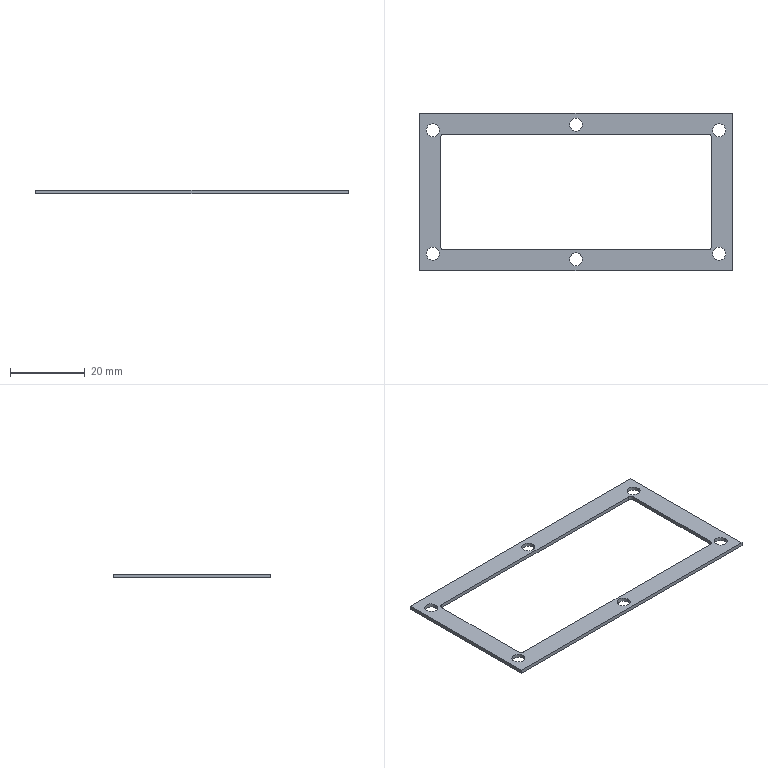Part | SolidWorks | features Extrusion 1, Fillet 1 | 1 solid | 26 faces | box 83.5 x 42 x 1 mm | volume 1203 mm3 | cylinder 16 | plane 10 | commonest cylinder face diameters 3.5 x12 2 x4
STEP:
#1=CARTESIAN_POINT('',(-1.75,-18.,1.));
#2=VERTEX_POINT('',#1);
#3=CARTESIAN_POINT('',(1.75,-18.,1.));
#4=VERTEX_POINT('',#3);
#5=CARTESIAN_POINT('',(0.,-18.,1.));
#6=DIRECTION('',(0.,0.,1.));
#7=DIRECTION('',(1.,0.,0.));
#8=AXIS2_PLACEMENT_3D('',#5,#6,#7);
#9=CIRCLE('',#8,1.75);
#10=EDGE_CURVE('',#2,#4,#9,.T.);
#11=ORIENTED_EDGE('',*,*,#10,.T.);
#12=CARTESIAN_POINT('',(1.75,-18.,0.));
#13=VERTEX_POINT('',#12);
#14=CARTESIAN_POINT('',(1.75,-18.,1.));
#15=DIRECTION('',(0.,0.,-1.));
#16=VECTOR('',#15,1000.);
#17=LINE('',#14,#16);
#18=EDGE_CURVE('',#4,#13,#17,.T.);
#19=ORIENTED_EDGE('',*,*,#18,.T.);
#20=CARTESIAN_POINT('',(-1.75,-18.,0.));
#21=VERTEX_POINT('',#20);
#22=CARTESIAN_POINT('',(0.,-18.,0.));
#23=DIRECTION('',(0.,0.,1.));
#24=DIRECTION('',(1.,0.,0.));
#25=AXIS2_PLACEMENT_3D('',#22,#23,#24);
#26=CIRCLE('',#25,1.75);
#27=EDGE_CURVE('',#21,#13,#26,.T.);
#28=ORIENTED_EDGE('',*,*,#27,.F.);
#29=CARTESIAN_POINT('',(-1.75,-18.,1.));
#30=DIRECTION('',(0.,0.,-1.));
#31=VECTOR('',#30,1000.);
#32=LINE('',#29,#31);
#33=EDGE_CURVE('',#2,#21,#32,.T.);
#34=ORIENTED_EDGE('',*,*,#33,.F.);
#35=EDGE_LOOP('',(#11,#19,#28,#34));
#36=FACE_OUTER_BOUND('',#35,.T.);
#37=CARTESIAN_POINT('',(0.,-18.,1.));
#38=DIRECTION('',(0.,0.,-1.));
#39=DIRECTION('',(-1.,0.,0.));
#40=AXIS2_PLACEMENT_3D('',#37,#38,#39);
#41=CYLINDRICAL_SURFACE('',#40,1.75);
#42=ADVANCED_FACE('',(#36),#41,.F.);
#43=CARTESIAN_POINT('',(-1.75,18.,1.));
#44=VERTEX_POINT('',#43);
#45=CARTESIAN_POINT('',(1.75,18.,1.));
#46=VERTEX_POINT('',#45);
#47=CARTESIAN_POINT('',(0.,18.,1.));
#48=DIRECTION('',(0.,0.,1.));
#49=DIRECTION('',(1.,0.,0.));
#50=AXIS2_PLACEMENT_3D('',#47,#48,#49);
#51=CIRCLE('',#50,1.75);
#52=EDGE_CURVE('',#44,#46,#51,.T.);
#53=ORIENTED_EDGE('',*,*,#52,.T.);
#54=CARTESIAN_POINT('',(1.75,18.,0.));
#55=VERTEX_POINT('',#54);
#56=CARTESIAN_POINT('',(1.75,18.,1.));
#57=DIRECTION('',(0.,0.,-1.));
#58=VECTOR('',#57,1000.);
#59=LINE('',#56,#58);
#60=EDGE_CURVE('',#46,#55,#59,.T.);
#61=ORIENTED_EDGE('',*,*,#60,.T.);
#62=CARTESIAN_POINT('',(-1.75,18.,0.));
#63=VERTEX_POINT('',#62);
#64=CARTESIAN_POINT('',(0.,18.,0.));
#65=DIRECTION('',(0.,0.,1.));
#66=DIRECTION('',(1.,0.,0.));
#67=AXIS2_PLACEMENT_3D('',#64,#65,#66);
#68=CIRCLE('',#67,1.75);
#69=EDGE_CURVE('',#63,#55,#68,.T.);
#70=ORIENTED_EDGE('',*,*,#69,.F.);
#71=CARTESIAN_POINT('',(-1.75,18.,1.));
#72=DIRECTION('',(0.,0.,-1.));
#73=VECTOR('',#72,1000.);
#74=LINE('',#71,#73);
#75=EDGE_CURVE('',#44,#63,#74,.T.);
#76=ORIENTED_EDGE('',*,*,#75,.F.);
#77=EDGE_LOOP('',(#53,#61,#70,#76));
#78=FACE_OUTER_BOUND('',#77,.T.);
#79=CARTESIAN_POINT('',(0.,18.,1.));
#80=DIRECTION('',(0.,0.,-1.));
#81=DIRECTION('',(-1.,0.,0.));
#82=AXIS2_PLACEMENT_3D('',#79,#80,#81);
#83=CYLINDRICAL_SURFACE('',#82,1.75);
#84=ADVANCED_FACE('',(#78),#83,.F.);
#85=CARTESIAN_POINT('',(-40.,-16.5,1.));
#86=VERTEX_POINT('',#85);
#87=CARTESIAN_POINT('',(-36.5,-16.5,1.));
#88=VERTEX_POINT('',#87);
#89=CARTESIAN_POINT('',(-38.25,-16.5,1.));
#90=DIRECTION('',(0.,0.,1.));
#91=DIRECTION('',(1.,0.,0.));
#92=AXIS2_PLACEMENT_3D('',#89,#90,#91);
#93=CIRCLE('',#92,1.75);
#94=EDGE_CURVE('',#86,#88,#93,.T.);
#95=ORIENTED_EDGE('',*,*,#94,.T.);
#96=CARTESIAN_POINT('',(-36.5,-16.5,0.));
#97=VERTEX_POINT('',#96);
#98=CARTESIAN_POINT('',(-36.5,-16.5,1.));
#99=DIRECTION('',(0.,0.,-1.));
#100=VECTOR('',#99,1000.);
#101=LINE('',#98,#100);
#102=EDGE_CURVE('',#88,#97,#101,.T.);
#103=ORIENTED_EDGE('',*,*,#102,.T.);
#104=CARTESIAN_POINT('',(-40.,-16.5,0.));
#105=VERTEX_POINT('',#104);
#106=CARTESIAN_POINT('',(-38.25,-16.5,0.));
#107=DIRECTION('',(0.,0.,1.));
#108=DIRECTION('',(1.,0.,0.));
#109=AXIS2_PLACEMENT_3D('',#106,#107,#108);
#110=CIRCLE('',#109,1.75);
#111=EDGE_CURVE('',#105,#97,#110,.T.);
#112=ORIENTED_EDGE('',*,*,#111,.F.);
#113=CARTESIAN_POINT('',(-40.,-16.5,1.));
#114=DIRECTION('',(0.,0.,-1.));
#115=VECTOR('',#114,1000.);
#116=LINE('',#113,#115);
#117=EDGE_CURVE('',#86,#105,#116,.T.);
#118=ORIENTED_EDGE('',*,*,#117,.F.);
#119=EDGE_LOOP('',(#95,#103,#112,#118));
#120=FACE_OUTER_BOUND('',#119,.T.);
#121=CARTESIAN_POINT('',(-38.25,-16.5,1.));
#122=DIRECTION('',(0.,0.,-1.));
#123=DIRECTION('',(-1.,0.,0.));
#124=AXIS2_PLACEMENT_3D('',#121,#122,#123);
#125=CYLINDRICAL_SURFACE('',#124,1.75);
#126=ADVANCED_FACE('',(#120),#125,.F.);
#127=CARTESIAN_POINT('',(36.5,-16.5,1.));
#128=VERTEX_POINT('',#127);
#129=CARTESIAN_POINT('',(40.,-16.5,1.));
#130=VERTEX_POINT('',#129);
#131=CARTESIAN_POINT('',(38.25,-16.5,1.));
#132=DIRECTION('',(0.,0.,1.));
#133=DIRECTION('',(1.,0.,0.));
#134=AXIS2_PLACEMENT_3D('',#131,#132,#133);
#135=CIRCLE('',#134,1.75);
#136=EDGE_CURVE('',#128,#130,#135,.T.);
#137=ORIENTED_EDGE('',*,*,#136,.T.);
#138=CARTESIAN_POINT('',(40.,-16.5,0.));
#139=VERTEX_POINT('',#138);
#140=CARTESIAN_POINT('',(40.,-16.5,1.));
#141=DIRECTION('',(0.,0.,-1.));
#142=VECTOR('',#141,1000.);
#143=LINE('',#140,#142);
#144=EDGE_CURVE('',#130,#139,#143,.T.);
#145=ORIENTED_EDGE('',*,*,#144,.T.);
#146=CARTESIAN_POINT('',(36.5,-16.5,0.));
#147=VERTEX_POINT('',#146);
#148=CARTESIAN_POINT('',(38.25,-16.5,0.));
#149=DIRECTION('',(0.,0.,1.));
#150=DIRECTION('',(1.,0.,0.));
#151=AXIS2_PLACEMENT_3D('',#148,#149,#150);
#152=CIRCLE('',#151,1.75);
#153=EDGE_CURVE('',#147,#139,#152,.T.);
#154=ORIENTED_EDGE('',*,*,#153,.F.);
#155=CARTESIAN_POINT('',(36.5,-16.5,1.));
#156=DIRECTION('',(0.,0.,-1.));
#157=VECTOR('',#156,1000.);
#158=LINE('',#155,#157);
#159=EDGE_CURVE('',#128,#147,#158,.T.);
#160=ORIENTED_EDGE('',*,*,#159,.F.);
#161=EDGE_LOOP('',(#137,#145,#154,#160));
#162=FACE_OUTER_BOUND('',#161,.T.);
#163=CARTESIAN_POINT('',(38.25,-16.5,1.));
#164=DIRECTION('',(0.,0.,-1.));
#165=DIRECTION('',(-1.,0.,0.));
#166=AXIS2_PLACEMENT_3D('',#163,#164,#165);
#167=CYLINDRICAL_SURFACE('',#166,1.75);
#168=ADVANCED_FACE('',(#162),#167,.F.);
#169=CARTESIAN_POINT('',(36.5,16.5,1.));
#170=VERTEX_POINT('',#169);
#171=CARTESIAN_POINT('',(40.,16.5,1.));
#172=VERTEX_POINT('',#171);
#173=CARTESIAN_POINT('',(38.25,16.5,1.));
#174=DIRECTION('',(0.,0.,1.));
#175=DIRECTION('',(1.,0.,0.));
#176=AXIS2_PLACEMENT_3D('',#173,#174,#175);
#177=CIRCLE('',#176,1.75);
#178=EDGE_CURVE('',#170,#172,#177,.T.);
#179=ORIENTED_EDGE('',*,*,#178,.T.);
#180=CARTESIAN_POINT('',(40.,16.5,0.));
#181=VERTEX_POINT('',#180);
#182=CARTESIAN_POINT('',(40.,16.5,1.));
#183=DIRECTION('',(0.,0.,-1.));
#184=VECTOR('',#183,1000.);
#185=LINE('',#182,#184);
#186=EDGE_CURVE('',#172,#181,#185,.T.);
#187=ORIENTED_EDGE('',*,*,#186,.T.);
#188=CARTESIAN_POINT('',(36.5,16.5,0.));
#189=VERTEX_POINT('',#188);
#190=CARTESIAN_POINT('',(38.25,16.5,0.));
#191=DIRECTION('',(0.,0.,1.));
#192=DIRECTION('',(1.,0.,0.));
#193=AXIS2_PLACEMENT_3D('',#190,#191,#192);
#194=CIRCLE('',#193,1.75);
#195=EDGE_CURVE('',#189,#181,#194,.T.);
#196=ORIENTED_EDGE('',*,*,#195,.F.);
#197=CARTESIAN_POINT('',(36.5,16.5,1.));
#198=DIRECTION('',(0.,0.,-1.));
#199=VECTOR('',#198,1000.);
#200=LINE('',#197,#199);
#201=EDGE_CURVE('',#170,#189,#200,.T.);
#202=ORIENTED_EDGE('',*,*,#201,.F.);
#203=EDGE_LOOP('',(#179,#187,#196,#202));
#204=FACE_OUTER_BOUND('',#203,.T.);
#205=CARTESIAN_POINT('',(38.25,16.5,1.));
#206=DIRECTION('',(0.,0.,-1.));
#207=DIRECTION('',(-1.,0.,0.));
#208=AXIS2_PLACEMENT_3D('',#205,#206,#207);
#209=CYLINDRICAL_SURFACE('',#208,1.75);
#210=ADVANCED_FACE('',(#204),#209,.F.);
#211=CARTESIAN_POINT('',(-40.,16.5,1.));
#212=VERTEX_POINT('',#211);
#213=CARTESIAN_POINT('',(-36.5,16.5,1.));
#214=VERTEX_POINT('',#213);
#215=CARTESIAN_POINT('',(-38.25,16.5,1.));
#216=DIRECTION('',(0.,0.,1.));
#217=DIRECTION('',(1.,0.,0.));
#218=AXIS2_PLACEMENT_3D('',#215,#216,#217);
#219=CIRCLE('',#218,1.75);
#220=EDGE_CURVE('',#212,#214,#219,.T.);
#221=ORIENTED_EDGE('',*,*,#220,.T.);
#222=CARTESIAN_POINT('',(-36.5,16.5,0.));
#223=VERTEX_POINT('',#222);
#224=CARTESIAN_POINT('',(-36.5,16.5,1.));
#225=DIRECTION('',(0.,0.,-1.));
#226=VECTOR('',#225,1000.);
#227=LINE('',#224,#226);
#228=EDGE_CURVE('',#214,#223,#227,.T.);
#229=ORIENTED_EDGE('',*,*,#228,.T.);
#230=CARTESIAN_POINT('',(-40.,16.5,0.));
#231=VERTEX_POINT('',#230);
#232=CARTESIAN_POINT('',(-38.25,16.5,0.));
#233=DIRECTION('',(0.,0.,1.));
#234=DIRECTION('',(1.,0.,0.));
#235=AXIS2_PLACEMENT_3D('',#232,#233,#234);
#236=CIRCLE('',#235,1.75);
#237=EDGE_CURVE('',#231,#223,#236,.T.);
#238=ORIENTED_EDGE('',*,*,#237,.F.);
#239=CARTESIAN_POINT('',(-40.,16.5,1.));
#240=DIRECTION('',(0.,0.,-1.));
#241=VECTOR('',#240,1000.);
#242=LINE('',#239,#241);
#243=EDGE_CURVE('',#212,#231,#242,.T.);
#244=ORIENTED_EDGE('',*,*,#243,.F.);
#245=EDGE_LOOP('',(#221,#229,#238,#244));
#246=FACE_OUTER_BOUND('',#245,.T.);
#247=CARTESIAN_POINT('',(-38.25,16.5,1.));
#248=DIRECTION('',(0.,0.,-1.));
#249=DIRECTION('',(-1.,0.,0.));
#250=AXIS2_PLACEMENT_3D('',#247,#248,#249);
#251=CYLINDRICAL_SURFACE('',#250,1.75);
#252=ADVANCED_FACE('',(#246),#251,.F.);
#253=ORIENTED_EDGE('',*,*,#52,.F.);
#254=CARTESIAN_POINT('',(0.,18.,1.));
#255=DIRECTION('',(0.,0.,1.));
#256=DIRECTION('',(1.,0.,0.));
#257=AXIS2_PLACEMENT_3D('',#254,#255,#256);
#258=CIRCLE('',#257,1.75);
#259=EDGE_CURVE('',#46,#44,#258,.T.);
#260=ORIENTED_EDGE('',*,*,#259,.F.);
#261=EDGE_LOOP('',(#253,#260));
#262=FACE_BOUND('',#261,.T.);
#263=ORIENTED_EDGE('',*,*,#136,.F.);
#264=CARTESIAN_POINT('',(38.25,-16.5,1.));
#265=DIRECTION('',(0.,0.,1.));
#266=DIRECTION('',(1.,0.,0.));
#267=AXIS2_PLACEMENT_3D('',#264,#265,#266);
#268=CIRCLE('',#267,1.75);
#269=EDGE_CURVE('',#130,#128,#268,.T.);
#270=ORIENTED_EDGE('',*,*,#269,.F.);
#271=EDGE_LOOP('',(#263,#270));
#272=FACE_BOUND('',#271,.T.);
#273=ORIENTED_EDGE('',*,*,#220,.F.);
#274=CARTESIAN_POINT('',(-38.25,16.5,1.));
#275=DIRECTION('',(0.,0.,1.));
#276=DIRECTION('',(1.,0.,0.));
#277=AXIS2_PLACEMENT_3D('',#274,#275,#276);
#278=CIRCLE('',#277,1.75);
#279=EDGE_CURVE('',#214,#212,#278,.T.);
#280=ORIENTED_EDGE('',*,*,#279,.F.);
#281=EDGE_LOOP('',(#273,#280));
#282=FACE_BOUND('',#281,.T.);
#283=CARTESIAN_POINT('',(-41.75,21.,1.));
#284=VERTEX_POINT('',#283);
#285=CARTESIAN_POINT('',(-41.75,-21.,1.));
#286=VERTEX_POINT('',#285);
#287=CARTESIAN_POINT('',(-41.75,-21.,1.));
#288=DIRECTION('',(0.,-1.,0.));
#289=VECTOR('',#288,1000.);
#290=LINE('',#287,#289);
#291=EDGE_CURVE('',#284,#286,#290,.T.);
#292=ORIENTED_EDGE('',*,*,#291,.T.);
#293=CARTESIAN_POINT('',(41.75,-21.,1.));
#294=VERTEX_POINT('',#293);
#295=CARTESIAN_POINT('',(41.75,-21.,1.));
#296=DIRECTION('',(1.,0.,0.));
#297=VECTOR('',#296,1000.);
#298=LINE('',#295,#297);
#299=EDGE_CURVE('',#286,#294,#298,.T.);
#300=ORIENTED_EDGE('',*,*,#299,.T.);
#301=CARTESIAN_POINT('',(41.75,21.,1.));
#302=VERTEX_POINT('',#301);
#303=CARTESIAN_POINT('',(41.75,-21.,1.));
#304=DIRECTION('',(0.,1.,0.));
#305=VECTOR('',#304,1000.);
#306=LINE('',#303,#305);
#307=EDGE_CURVE('',#294,#302,#306,.T.);
#308=ORIENTED_EDGE('',*,*,#307,.T.);
#309=CARTESIAN_POINT('',(41.75,21.,1.));
#310=DIRECTION('',(-1.,0.,0.));
#311=VECTOR('',#310,1000.);
#312=LINE('',#309,#311);
#313=EDGE_CURVE('',#302,#284,#312,.T.);
#314=ORIENTED_EDGE('',*,*,#313,.T.);
#315=EDGE_LOOP('',(#292,#300,#308,#314));
#316=FACE_OUTER_BOUND('',#315,.T.);
#317=ORIENTED_EDGE('',*,*,#178,.F.);
#318=CARTESIAN_POINT('',(38.25,16.5,1.));
#319=DIRECTION('',(0.,0.,1.));
#320=DIRECTION('',(1.,0.,0.));
#321=AXIS2_PLACEMENT_3D('',#318,#319,#320);
#322=CIRCLE('',#321,1.75);
#323=EDGE_CURVE('',#172,#170,#322,.T.);
#324=ORIENTED_EDGE('',*,*,#323,.F.);
#325=EDGE_LOOP('',(#317,#324));
#326=FACE_BOUND('',#325,.T.);
#327=ORIENTED_EDGE('',*,*,#94,.F.);
#328=CARTESIAN_POINT('',(-38.25,-16.5,1.));
#329=DIRECTION('',(0.,0.,1.));
#330=DIRECTION('',(1.,0.,0.));
#331=AXIS2_PLACEMENT_3D('',#328,#329,#330);
#332=CIRCLE('',#331,1.75);
#333=EDGE_CURVE('',#88,#86,#332,.T.);
#334=ORIENTED_EDGE('',*,*,#333,.F.);
#335=EDGE_LOOP('',(#327,#334));
#336=FACE_BOUND('',#335,.T.);
#337=ORIENTED_EDGE('',*,*,#10,.F.);
#338=CARTESIAN_POINT('',(0.,-18.,1.));
#339=DIRECTION('',(0.,0.,1.));
#340=DIRECTION('',(1.,0.,0.));
#341=AXIS2_PLACEMENT_3D('',#338,#339,#340);
#342=CIRCLE('',#341,1.75);
#343=EDGE_CURVE('',#4,#2,#342,.T.);
#344=ORIENTED_EDGE('',*,*,#343,.F.);
#345=EDGE_LOOP('',(#337,#344));
#346=FACE_BOUND('',#345,.T.);
#347=CARTESIAN_POINT('',(-35.25,-15.5,1.));
#348=VERTEX_POINT('',#347);
#349=CARTESIAN_POINT('',(35.25,-15.5,1.));
#350=VERTEX_POINT('',#349);
#351=CARTESIAN_POINT('',(36.25,-15.5,1.));
#352=DIRECTION('',(1.,0.,0.));
#353=VECTOR('',#352,1000.);
#354=LINE('',#351,#353);
#355=EDGE_CURVE('',#348,#350,#354,.T.);
#356=ORIENTED_EDGE('',*,*,#355,.F.);
#357=CARTESIAN_POINT('',(-36.25,-14.5,1.));
#358=VERTEX_POINT('',#357);
#359=CARTESIAN_POINT('',(-35.25,-14.5,1.));
#360=DIRECTION('',(0.,0.,-1.));
#361=DIRECTION('',(1.,0.,0.));
#362=AXIS2_PLACEMENT_3D('',#359,#360,#361);
#363=CIRCLE('',#362,1.);
#364=EDGE_CURVE('',#348,#358,#363,.T.);
#365=ORIENTED_EDGE('',*,*,#364,.T.);
#366=CARTESIAN_POINT('',(-36.25,14.5,1.));
#367=VERTEX_POINT('',#366);
#368=CARTESIAN_POINT('',(-36.25,-15.5,1.));
#369=DIRECTION('',(0.,-1.,0.));
#370=VECTOR('',#369,1000.);
#371=LINE('',#368,#370);
#372=EDGE_CURVE('',#367,#358,#371,.T.);
#373=ORIENTED_EDGE('',*,*,#372,.F.);
#374=CARTESIAN_POINT('',(-35.25,15.5,1.));
#375=VERTEX_POINT('',#374);
#376=CARTESIAN_POINT('',(-35.25,14.5,1.));
#377=DIRECTION('',(0.,0.,-1.));
#378=DIRECTION('',(1.,0.,0.));
#379=AXIS2_PLACEMENT_3D('',#376,#377,#378);
#380=CIRCLE('',#379,1.);
#381=EDGE_CURVE('',#367,#375,#380,.T.);
#382=ORIENTED_EDGE('',*,*,#381,.T.);
#383=CARTESIAN_POINT('',(35.25,15.5,1.));
#384=VERTEX_POINT('',#383);
#385=CARTESIAN_POINT('',(36.25,15.5,1.));
#386=DIRECTION('',(-1.,0.,0.));
#387=VECTOR('',#386,1000.);
#388=LINE('',#385,#387);
#389=EDGE_CURVE('',#384,#375,#388,.T.);
#390=ORIENTED_EDGE('',*,*,#389,.F.);
#391=CARTESIAN_POINT('',(36.25,14.5,1.));
#392=VERTEX_POINT('',#391);
#393=CARTESIAN_POINT('',(35.25,14.5,1.));
#394=DIRECTION('',(0.,0.,-1.));
#395=DIRECTION('',(1.,0.,0.));
#396=AXIS2_PLACEMENT_3D('',#393,#394,#395);
#397=CIRCLE('',#396,1.);
#398=EDGE_CURVE('',#384,#392,#397,.T.);
#399=ORIENTED_EDGE('',*,*,#398,.T.);
#400=CARTESIAN_POINT('',(36.25,-14.5,1.));
#401=VERTEX_POINT('',#400);
#402=CARTESIAN_POINT('',(36.25,-15.5,1.));
#403=DIRECTION('',(0.,1.,0.));
#404=VECTOR('',#403,1000.);
#405=LINE('',#402,#404);
#406=EDGE_CURVE('',#401,#392,#405,.T.);
#407=ORIENTED_EDGE('',*,*,#406,.F.);
#408=CARTESIAN_POINT('',(35.25,-14.5,1.));
#409=DIRECTION('',(0.,0.,-1.));
#410=DIRECTION('',(1.,0.,0.));
#411=AXIS2_PLACEMENT_3D('',#408,#409,#410);
#412=CIRCLE('',#411,1.);
#413=EDGE_CURVE('',#401,#350,#412,.T.);
#414=ORIENTED_EDGE('',*,*,#413,.T.);
#415=EDGE_LOOP('',(#356,#365,#373,#382,#390,#399,#407,#414));
#416=FACE_BOUND('',#415,.T.);
#417=CARTESIAN_POINT('',(0.,0.,1.));
#418=DIRECTION('',(0.,0.,1.));
#419=DIRECTION('',(1.,0.,0.));
#420=AXIS2_PLACEMENT_3D('',#417,#418,#419);
#421=PLANE('',#420);
#422=ADVANCED_FACE('',(#262,#272,#282,#316,#326,#336,#346,#416),#421,.T.);
#423=ORIENTED_EDGE('',*,*,#27,.T.);
#424=CARTESIAN_POINT('',(0.,-18.,0.));
#425=DIRECTION('',(0.,0.,1.));
#426=DIRECTION('',(1.,0.,0.));
#427=AXIS2_PLACEMENT_3D('',#424,#425,#426);
#428=CIRCLE('',#427,1.75);
#429=EDGE_CURVE('',#13,#21,#428,.T.);
#430=ORIENTED_EDGE('',*,*,#429,.T.);
#431=EDGE_LOOP('',(#423,#430));
#432=FACE_BOUND('',#431,.T.);
#433=ORIENTED_EDGE('',*,*,#69,.T.);
#434=CARTESIAN_POINT('',(0.,18.,0.));
#435=DIRECTION('',(0.,0.,1.));
#436=DIRECTION('',(1.,0.,0.));
#437=AXIS2_PLACEMENT_3D('',#434,#435,#436);
#438=CIRCLE('',#437,1.75);
#439=EDGE_CURVE('',#55,#63,#438,.T.);
#440=ORIENTED_EDGE('',*,*,#439,.T.);
#441=EDGE_LOOP('',(#433,#440));
#442=FACE_BOUND('',#441,.T.);
#443=ORIENTED_EDGE('',*,*,#111,.T.);
#444=CARTESIAN_POINT('',(-38.25,-16.5,0.));
#445=DIRECTION('',(0.,0.,1.));
#446=DIRECTION('',(1.,0.,0.));
#447=AXIS2_PLACEMENT_3D('',#444,#445,#446);
#448=CIRCLE('',#447,1.75);
#449=EDGE_CURVE('',#97,#105,#448,.T.);
#450=ORIENTED_EDGE('',*,*,#449,.T.);
#451=EDGE_LOOP('',(#443,#450));
#452=FACE_BOUND('',#451,.T.);
#453=ORIENTED_EDGE('',*,*,#153,.T.);
#454=CARTESIAN_POINT('',(38.25,-16.5,0.));
#455=DIRECTION('',(0.,0.,1.));
#456=DIRECTION('',(1.,0.,0.));
#457=AXIS2_PLACEMENT_3D('',#454,#455,#456);
#458=CIRCLE('',#457,1.75);
#459=EDGE_CURVE('',#139,#147,#458,.T.);
#460=ORIENTED_EDGE('',*,*,#459,.T.);
#461=EDGE_LOOP('',(#453,#460));
#462=FACE_BOUND('',#461,.T.);
#463=ORIENTED_EDGE('',*,*,#195,.T.);
#464=CARTESIAN_POINT('',(38.25,16.5,0.));
#465=DIRECTION('',(0.,0.,1.));
#466=DIRECTION('',(1.,0.,0.));
#467=AXIS2_PLACEMENT_3D('',#464,#465,#466);
#468=CIRCLE('',#467,1.75);
#469=EDGE_CURVE('',#181,#189,#468,.T.);
#470=ORIENTED_EDGE('',*,*,#469,.T.);
#471=EDGE_LOOP('',(#463,#470));
#472=FACE_BOUND('',#471,.T.);
#473=ORIENTED_EDGE('',*,*,#237,.T.);
#474=CARTESIAN_POINT('',(-38.25,16.5,0.));
#475=DIRECTION('',(0.,0.,1.));
#476=DIRECTION('',(1.,0.,0.));
#477=AXIS2_PLACEMENT_3D('',#474,#475,#476);
#478=CIRCLE('',#477,1.75);
#479=EDGE_CURVE('',#223,#231,#478,.T.);
#480=ORIENTED_EDGE('',*,*,#479,.T.);
#481=EDGE_LOOP('',(#473,#480));
#482=FACE_BOUND('',#481,.T.);
#483=CARTESIAN_POINT('',(-41.75,21.,0.));
#484=VERTEX_POINT('',#483);
#485=CARTESIAN_POINT('',(-41.75,-21.,0.));
#486=VERTEX_POINT('',#485);
#487=CARTESIAN_POINT('',(-41.75,-21.,0.));
#488=DIRECTION('',(0.,-1.,0.));
#489=VECTOR('',#488,1000.);
#490=LINE('',#487,#489);
#491=EDGE_CURVE('',#484,#486,#490,.T.);
#492=ORIENTED_EDGE('',*,*,#491,.F.);
#493=CARTESIAN_POINT('',(41.75,21.,0.));
#494=VERTEX_POINT('',#493);
#495=CARTESIAN_POINT('',(41.75,21.,0.));
#496=DIRECTION('',(-1.,0.,0.));
#497=VECTOR('',#496,1000.);
#498=LINE('',#495,#497);
#499=EDGE_CURVE('',#494,#484,#498,.T.);
#500=ORIENTED_EDGE('',*,*,#499,.F.);
#501=CARTESIAN_POINT('',(41.75,-21.,0.));
#502=VERTEX_POINT('',#501);
#503=CARTESIAN_POINT('',(41.75,-21.,0.));
#504=DIRECTION('',(0.,1.,0.));
#505=VECTOR('',#504,1000.);
#506=LINE('',#503,#505);
#507=EDGE_CURVE('',#502,#494,#506,.T.);
#508=ORIENTED_EDGE('',*,*,#507,.F.);
#509=CARTESIAN_POINT('',(41.75,-21.,0.));
#510=DIRECTION('',(1.,0.,0.));
#511=VECTOR('',#510,1000.);
#512=LINE('',#509,#511);
#513=EDGE_CURVE('',#486,#502,#512,.T.);
#514=ORIENTED_EDGE('',*,*,#513,.F.);
#515=EDGE_LOOP('',(#492,#500,#508,#514));
#516=FACE_OUTER_BOUND('',#515,.T.);
#517=CARTESIAN_POINT('',(35.25,15.5,0.));
#518=VERTEX_POINT('',#517);
#519=CARTESIAN_POINT('',(-35.25,15.5,0.));
#520=VERTEX_POINT('',#519);
#521=CARTESIAN_POINT('',(36.25,15.5,0.));
#522=DIRECTION('',(-1.,0.,0.));
#523=VECTOR('',#522,1000.);
#524=LINE('',#521,#523);
#525=EDGE_CURVE('',#518,#520,#524,.T.);
#526=ORIENTED_EDGE('',*,*,#525,.T.);
#527=CARTESIAN_POINT('',(-36.25,14.5,0.));
#528=VERTEX_POINT('',#527);
#529=CARTESIAN_POINT('',(-35.25,14.5,0.));
#530=DIRECTION('',(0.,0.,1.));
#531=DIRECTION('',(1.,0.,0.));
#532=AXIS2_PLACEMENT_3D('',#529,#530,#531);
#533=CIRCLE('',#532,1.);
#534=EDGE_CURVE('',#520,#528,#533,.T.);
#535=ORIENTED_EDGE('',*,*,#534,.T.);
#536=CARTESIAN_POINT('',(-36.25,-14.5,0.));
#537=VERTEX_POINT('',#536);
#538=CARTESIAN_POINT('',(-36.25,-15.5,0.));
#539=DIRECTION('',(0.,-1.,0.));
#540=VECTOR('',#539,1000.);
#541=LINE('',#538,#540);
#542=EDGE_CURVE('',#528,#537,#541,.T.);
#543=ORIENTED_EDGE('',*,*,#542,.T.);
#544=CARTESIAN_POINT('',(-35.25,-15.5,0.));
#545=VERTEX_POINT('',#544);
#546=CARTESIAN_POINT('',(-35.25,-14.5,0.));
#547=DIRECTION('',(0.,0.,1.));
#548=DIRECTION('',(1.,0.,0.));
#549=AXIS2_PLACEMENT_3D('',#546,#547,#548);
#550=CIRCLE('',#549,1.);
#551=EDGE_CURVE('',#537,#545,#550,.T.);
#552=ORIENTED_EDGE('',*,*,#551,.T.);
#553=CARTESIAN_POINT('',(35.25,-15.5,0.));
#554=VERTEX_POINT('',#553);
#555=CARTESIAN_POINT('',(36.25,-15.5,0.));
#556=DIRECTION('',(1.,0.,0.));
#557=VECTOR('',#556,1000.);
#558=LINE('',#555,#557);
#559=EDGE_CURVE('',#545,#554,#558,.T.);
#560=ORIENTED_EDGE('',*,*,#559,.T.);
#561=CARTESIAN_POINT('',(36.25,-14.5,0.));
#562=VERTEX_POINT('',#561);
#563=CARTESIAN_POINT('',(35.25,-14.5,0.));
#564=DIRECTION('',(0.,0.,1.));
#565=DIRECTION('',(1.,0.,0.));
#566=AXIS2_PLACEMENT_3D('',#563,#564,#565);
#567=CIRCLE('',#566,1.);
#568=EDGE_CURVE('',#554,#562,#567,.T.);
#569=ORIENTED_EDGE('',*,*,#568,.T.);
#570=CARTESIAN_POINT('',(36.25,14.5,0.));
#571=VERTEX_POINT('',#570);
#572=CARTESIAN_POINT('',(36.25,-15.5,0.));
#573=DIRECTION('',(0.,1.,0.));
#574=VECTOR('',#573,1000.);
#575=LINE('',#572,#574);
#576=EDGE_CURVE('',#562,#571,#575,.T.);
#577=ORIENTED_EDGE('',*,*,#576,.T.);
#578=CARTESIAN_POINT('',(35.25,14.5,0.));
#579=DIRECTION('',(0.,0.,1.));
#580=DIRECTION('',(1.,0.,0.));
#581=AXIS2_PLACEMENT_3D('',#578,#579,#580);
#582=CIRCLE('',#581,1.);
#583=EDGE_CURVE('',#571,#518,#582,.T.);
#584=ORIENTED_EDGE('',*,*,#583,.T.);
#585=EDGE_LOOP('',(#526,#535,#543,#552,#560,#569,#577,#584));
#586=FACE_BOUND('',#585,.T.);
#587=CARTESIAN_POINT('',(0.,0.,0.));
#588=DIRECTION('',(0.,0.,1.));
#589=DIRECTION('',(1.,0.,0.));
#590=AXIS2_PLACEMENT_3D('',#587,#588,#589);
#591=PLANE('',#590);
#592=ADVANCED_FACE('',(#432,#442,#452,#462,#472,#482,#516,#586),#591,.F.);
#593=ORIENTED_EDGE('',*,*,#491,.T.);
#594=CARTESIAN_POINT('',(-41.75,-21.,1.));
#595=DIRECTION('',(0.,0.,-1.));
#596=VECTOR('',#595,1000.);
#597=LINE('',#594,#596);
#598=EDGE_CURVE('',#286,#486,#597,.T.);
#599=ORIENTED_EDGE('',*,*,#598,.F.);
#600=ORIENTED_EDGE('',*,*,#291,.F.);
#601=CARTESIAN_POINT('',(-41.75,21.,1.));
#602=DIRECTION('',(0.,0.,-1.));
#603=VECTOR('',#602,1000.);
#604=LINE('',#601,#603);
#605=EDGE_CURVE('',#284,#484,#604,.T.);
#606=ORIENTED_EDGE('',*,*,#605,.T.);
#607=EDGE_LOOP('',(#593,#599,#600,#606));
#608=FACE_OUTER_BOUND('',#607,.T.);
#609=CARTESIAN_POINT('',(-41.75,-21.,1.));
#610=DIRECTION('',(1.,0.,0.));
#611=DIRECTION('',(0.,0.,-1.));
#612=AXIS2_PLACEMENT_3D('',#609,#610,#611);
#613=PLANE('',#612);
#614=ADVANCED_FACE('',(#608),#613,.F.);
#615=ORIENTED_EDGE('',*,*,#513,.T.);
#616=CARTESIAN_POINT('',(41.75,-21.,1.));
#617=DIRECTION('',(0.,0.,-1.));
#618=VECTOR('',#617,1000.);
#619=LINE('',#616,#618);
#620=EDGE_CURVE('',#294,#502,#619,.T.);
#621=ORIENTED_EDGE('',*,*,#620,.F.);
#622=ORIENTED_EDGE('',*,*,#299,.F.);
#623=ORIENTED_EDGE('',*,*,#598,.T.);
#624=EDGE_LOOP('',(#615,#621,#622,#623));
#625=FACE_OUTER_BOUND('',#624,.T.);
#626=CARTESIAN_POINT('',(41.75,-21.,1.));
#627=DIRECTION('',(0.,1.,0.));
#628=DIRECTION('',(-1.,0.,0.));
#629=AXIS2_PLACEMENT_3D('',#626,#627,#628);
#630=PLANE('',#629);
#631=ADVANCED_FACE('',(#625),#630,.F.);
#632=ORIENTED_EDGE('',*,*,#507,.T.);
#633=CARTESIAN_POINT('',(41.75,21.,1.));
#634=DIRECTION('',(0.,0.,-1.));
#635=VECTOR('',#634,1000.);
#636=LINE('',#633,#635);
#637=EDGE_CURVE('',#302,#494,#636,.T.);
#638=ORIENTED_EDGE('',*,*,#637,.F.);
#639=ORIENTED_EDGE('',*,*,#307,.F.);
#640=ORIENTED_EDGE('',*,*,#620,.T.);
#641=EDGE_LOOP('',(#632,#638,#639,#640));
#642=FACE_OUTER_BOUND('',#641,.T.);
#643=CARTESIAN_POINT('',(41.75,-21.,1.));
#644=DIRECTION('',(-1.,0.,0.));
#645=DIRECTION('',(0.,0.,1.));
#646=AXIS2_PLACEMENT_3D('',#643,#644,#645);
#647=PLANE('',#646);
#648=ADVANCED_FACE('',(#642),#647,.F.);
#649=ORIENTED_EDGE('',*,*,#499,.T.);
#650=ORIENTED_EDGE('',*,*,#605,.F.);
#651=ORIENTED_EDGE('',*,*,#313,.F.);
#652=ORIENTED_EDGE('',*,*,#637,.T.);
#653=EDGE_LOOP('',(#649,#650,#651,#652));
#654=FACE_OUTER_BOUND('',#653,.T.);
#655=CARTESIAN_POINT('',(41.75,21.,1.));
#656=DIRECTION('',(0.,-1.,0.));
#657=DIRECTION('',(1.,0.,0.));
#658=AXIS2_PLACEMENT_3D('',#655,#656,#657);
#659=PLANE('',#658);
#660=ADVANCED_FACE('',(#654),#659,.F.);
#661=ORIENTED_EDGE('',*,*,#228,.F.);
#662=ORIENTED_EDGE('',*,*,#279,.T.);
#663=ORIENTED_EDGE('',*,*,#243,.T.);
#664=ORIENTED_EDGE('',*,*,#479,.F.);
#665=EDGE_LOOP('',(#661,#662,#663,#664));
#666=FACE_OUTER_BOUND('',#665,.T.);
#667=CARTESIAN_POINT('',(-38.25,16.5,1.));
#668=DIRECTION('',(0.,0.,-1.));
#669=DIRECTION('',(-1.,0.,0.));
#670=AXIS2_PLACEMENT_3D('',#667,#668,#669);
#671=CYLINDRICAL_SURFACE('',#670,1.75);
#672=ADVANCED_FACE('',(#666),#671,.F.);
#673=ORIENTED_EDGE('',*,*,#186,.F.);
#674=ORIENTED_EDGE('',*,*,#323,.T.);
#675=ORIENTED_EDGE('',*,*,#201,.T.);
#676=ORIENTED_EDGE('',*,*,#469,.F.);
#677=EDGE_LOOP('',(#673,#674,#675,#676));
#678=FACE_OUTER_BOUND('',#677,.T.);
#679=CARTESIAN_POINT('',(38.25,16.5,1.));
#680=DIRECTION('',(0.,0.,-1.));
#681=DIRECTION('',(-1.,0.,0.));
#682=AXIS2_PLACEMENT_3D('',#679,#680,#681);
#683=CYLINDRICAL_SURFACE('',#682,1.75);
#684=ADVANCED_FACE('',(#678),#683,.F.);
#685=ORIENTED_EDGE('',*,*,#144,.F.);
#686=ORIENTED_EDGE('',*,*,#269,.T.);
#687=ORIENTED_EDGE('',*,*,#159,.T.);
#688=ORIENTED_EDGE('',*,*,#459,.F.);
#689=EDGE_LOOP('',(#685,#686,#687,#688));
#690=FACE_OUTER_BOUND('',#689,.T.);
#691=CARTESIAN_POINT('',(38.25,-16.5,1.));
#692=DIRECTION('',(0.,0.,-1.));
#693=DIRECTION('',(-1.,0.,0.));
#694=AXIS2_PLACEMENT_3D('',#691,#692,#693);
#695=CYLINDRICAL_SURFACE('',#694,1.75);
#696=ADVANCED_FACE('',(#690),#695,.F.);
#697=ORIENTED_EDGE('',*,*,#102,.F.);
#698=ORIENTED_EDGE('',*,*,#333,.T.);
#699=ORIENTED_EDGE('',*,*,#117,.T.);
#700=ORIENTED_EDGE('',*,*,#449,.F.);
#701=EDGE_LOOP('',(#697,#698,#699,#700));
#702=FACE_OUTER_BOUND('',#701,.T.);
#703=CARTESIAN_POINT('',(-38.25,-16.5,1.));
#704=DIRECTION('',(0.,0.,-1.));
#705=DIRECTION('',(-1.,0.,0.));
#706=AXIS2_PLACEMENT_3D('',#703,#704,#705);
#707=CYLINDRICAL_SURFACE('',#706,1.75);
#708=ADVANCED_FACE('',(#702),#707,.F.);
#709=ORIENTED_EDGE('',*,*,#60,.F.);
#710=ORIENTED_EDGE('',*,*,#259,.T.);
#711=ORIENTED_EDGE('',*,*,#75,.T.);
#712=ORIENTED_EDGE('',*,*,#439,.F.);
#713=EDGE_LOOP('',(#709,#710,#711,#712));
#714=FACE_OUTER_BOUND('',#713,.T.);
#715=CARTESIAN_POINT('',(0.,18.,1.));
#716=DIRECTION('',(0.,0.,-1.));
#717=DIRECTION('',(-1.,0.,0.));
#718=AXIS2_PLACEMENT_3D('',#715,#716,#717);
#719=CYLINDRICAL_SURFACE('',#718,1.75);
#720=ADVANCED_FACE('',(#714),#719,.F.);
#721=ORIENTED_EDGE('',*,*,#18,.F.);
#722=ORIENTED_EDGE('',*,*,#343,.T.);
#723=ORIENTED_EDGE('',*,*,#33,.T.);
#724=ORIENTED_EDGE('',*,*,#429,.F.);
#725=EDGE_LOOP('',(#721,#722,#723,#724));
#726=FACE_OUTER_BOUND('',#725,.T.);
#727=CARTESIAN_POINT('',(0.,-18.,1.));
#728=DIRECTION('',(0.,0.,-1.));
#729=DIRECTION('',(-1.,0.,0.));
#730=AXIS2_PLACEMENT_3D('',#727,#728,#729);
#731=CYLINDRICAL_SURFACE('',#730,1.75);
#732=ADVANCED_FACE('',(#726),#731,.F.);
#733=ORIENTED_EDGE('',*,*,#372,.T.);
#734=CARTESIAN_POINT('',(-36.25,-14.5,0.));
#735=DIRECTION('',(0.,0.,-1.));
#736=VECTOR('',#735,1000.);
#737=LINE('',#734,#736);
#738=EDGE_CURVE('',#358,#537,#737,.T.);
#739=ORIENTED_EDGE('',*,*,#738,.T.);
#740=ORIENTED_EDGE('',*,*,#542,.F.);
#741=CARTESIAN_POINT('',(-36.25,14.5,1.));
#742=DIRECTION('',(0.,0.,1.));
#743=VECTOR('',#742,1000.);
#744=LINE('',#741,#743);
#745=EDGE_CURVE('',#528,#367,#744,.T.);
#746=ORIENTED_EDGE('',*,*,#745,.T.);
#747=EDGE_LOOP('',(#733,#739,#740,#746));
#748=FACE_OUTER_BOUND('',#747,.T.);
#749=CARTESIAN_POINT('',(-36.25,-15.5,1.));
#750=DIRECTION('',(1.,0.,0.));
#751=DIRECTION('',(0.,0.,-1.));
#752=AXIS2_PLACEMENT_3D('',#749,#750,#751);
#753=PLANE('',#752);
#754=ADVANCED_FACE('',(#748),#753,.T.);
#755=ORIENTED_EDGE('',*,*,#355,.T.);
#756=CARTESIAN_POINT('',(35.25,-15.5,0.));
#757=DIRECTION('',(0.,0.,-1.));
#758=VECTOR('',#757,1000.);
#759=LINE('',#756,#758);
#760=EDGE_CURVE('',#350,#554,#759,.T.);
#761=ORIENTED_EDGE('',*,*,#760,.T.);
#762=ORIENTED_EDGE('',*,*,#559,.F.);
#763=CARTESIAN_POINT('',(-35.25,-15.5,1.));
#764=DIRECTION('',(0.,0.,1.));
#765=VECTOR('',#764,1000.);
#766=LINE('',#763,#765);
#767=EDGE_CURVE('',#545,#348,#766,.T.);
#768=ORIENTED_EDGE('',*,*,#767,.T.);
#769=EDGE_LOOP('',(#755,#761,#762,#768));
#770=FACE_OUTER_BOUND('',#769,.T.);
#771=CARTESIAN_POINT('',(36.25,-15.5,1.));
#772=DIRECTION('',(0.,1.,0.));
#773=DIRECTION('',(-1.,0.,0.));
#774=AXIS2_PLACEMENT_3D('',#771,#772,#773);
#775=PLANE('',#774);
#776=ADVANCED_FACE('',(#770),#775,.T.);
#777=ORIENTED_EDGE('',*,*,#406,.T.);
#778=CARTESIAN_POINT('',(36.25,14.5,0.));
#779=DIRECTION('',(0.,0.,-1.));
#780=VECTOR('',#779,1000.);
#781=LINE('',#778,#780);
#782=EDGE_CURVE('',#392,#571,#781,.T.);
#783=ORIENTED_EDGE('',*,*,#782,.T.);
#784=ORIENTED_EDGE('',*,*,#576,.F.);
#785=CARTESIAN_POINT('',(36.25,-14.5,1.));
#786=DIRECTION('',(0.,0.,1.));
#787=VECTOR('',#786,1000.);
#788=LINE('',#785,#787);
#789=EDGE_CURVE('',#562,#401,#788,.T.);
#790=ORIENTED_EDGE('',*,*,#789,.T.);
#791=EDGE_LOOP('',(#777,#783,#784,#790));
#792=FACE_OUTER_BOUND('',#791,.T.);
#793=CARTESIAN_POINT('',(36.25,-15.5,1.));
#794=DIRECTION('',(-1.,0.,0.));
#795=DIRECTION('',(0.,-1.,0.));
#796=AXIS2_PLACEMENT_3D('',#793,#794,#795);
#797=PLANE('',#796);
#798=ADVANCED_FACE('',(#792),#797,.T.);
#799=ORIENTED_EDGE('',*,*,#525,.F.);
#800=CARTESIAN_POINT('',(35.25,15.5,1.));
#801=DIRECTION('',(0.,0.,1.));
#802=VECTOR('',#801,1000.);
#803=LINE('',#800,#802);
#804=EDGE_CURVE('',#518,#384,#803,.T.);
#805=ORIENTED_EDGE('',*,*,#804,.T.);
#806=ORIENTED_EDGE('',*,*,#389,.T.);
#807=CARTESIAN_POINT('',(-35.25,15.5,0.));
#808=DIRECTION('',(0.,0.,-1.));
#809=VECTOR('',#808,1000.);
#810=LINE('',#807,#809);
#811=EDGE_CURVE('',#375,#520,#810,.T.);
#812=ORIENTED_EDGE('',*,*,#811,.T.);
#813=EDGE_LOOP('',(#799,#805,#806,#812));
#814=FACE_OUTER_BOUND('',#813,.T.);
#815=CARTESIAN_POINT('',(36.25,15.5,1.));
#816=DIRECTION('',(0.,-1.,0.));
#817=DIRECTION('',(1.,0.,0.));
#818=AXIS2_PLACEMENT_3D('',#815,#816,#817);
#819=PLANE('',#818);
#820=ADVANCED_FACE('',(#814),#819,.T.);
#821=ORIENTED_EDGE('',*,*,#398,.F.);
#822=ORIENTED_EDGE('',*,*,#804,.F.);
#823=ORIENTED_EDGE('',*,*,#583,.F.);
#824=ORIENTED_EDGE('',*,*,#782,.F.);
#825=EDGE_LOOP('',(#821,#822,#823,#824));
#826=FACE_OUTER_BOUND('',#825,.T.);
#827=CARTESIAN_POINT('',(35.25,14.5,1.));
#828=DIRECTION('',(0.,0.,1.));
#829=DIRECTION('',(1.,0.,0.));
#830=AXIS2_PLACEMENT_3D('',#827,#828,#829);
#831=CYLINDRICAL_SURFACE('',#830,1.);
#832=ADVANCED_FACE('',(#826),#831,.F.);
#833=ORIENTED_EDGE('',*,*,#413,.F.);
#834=ORIENTED_EDGE('',*,*,#789,.F.);
#835=ORIENTED_EDGE('',*,*,#568,.F.);
#836=ORIENTED_EDGE('',*,*,#760,.F.);
#837=EDGE_LOOP('',(#833,#834,#835,#836));
#838=FACE_OUTER_BOUND('',#837,.T.);
#839=CARTESIAN_POINT('',(35.25,-14.5,1.));
#840=DIRECTION('',(0.,0.,1.));
#841=DIRECTION('',(1.,0.,0.));
#842=AXIS2_PLACEMENT_3D('',#839,#840,#841);
#843=CYLINDRICAL_SURFACE('',#842,1.);
#844=ADVANCED_FACE('',(#838),#843,.F.);
#845=ORIENTED_EDGE('',*,*,#364,.F.);
#846=ORIENTED_EDGE('',*,*,#767,.F.);
#847=ORIENTED_EDGE('',*,*,#551,.F.);
#848=ORIENTED_EDGE('',*,*,#738,.F.);
#849=EDGE_LOOP('',(#845,#846,#847,#848));
#850=FACE_OUTER_BOUND('',#849,.T.);
#851=CARTESIAN_POINT('',(-35.25,-14.5,1.));
#852=DIRECTION('',(0.,0.,1.));
#853=DIRECTION('',(1.,0.,0.));
#854=AXIS2_PLACEMENT_3D('',#851,#852,#853);
#855=CYLINDRICAL_SURFACE('',#854,1.);
#856=ADVANCED_FACE('',(#850),#855,.F.);
#857=ORIENTED_EDGE('',*,*,#381,.F.);
#858=ORIENTED_EDGE('',*,*,#745,.F.);
#859=ORIENTED_EDGE('',*,*,#534,.F.);
#860=ORIENTED_EDGE('',*,*,#811,.F.);
#861=EDGE_LOOP('',(#857,#858,#859,#860));
#862=FACE_OUTER_BOUND('',#861,.T.);
#863=CARTESIAN_POINT('',(-35.25,14.5,1.));
#864=DIRECTION('',(0.,0.,1.));
#865=DIRECTION('',(1.,0.,0.));
#866=AXIS2_PLACEMENT_3D('',#863,#864,#865);
#867=CYLINDRICAL_SURFACE('',#866,1.);
#868=ADVANCED_FACE('',(#862),#867,.F.);
#869=CLOSED_SHELL('',(#42,#84,#126,#168,#210,#252,#422,#592,#614,#631,#648,#660,#672,#684,#696,#708,#720,#732,#754,#776,#798,#820,#832,#844,#856,#868));
#870=MANIFOLD_SOLID_BREP('',#869);
#871=CARTESIAN_POINT('',(0.,0.,0.));
#872=DIRECTION('',(0.,0.,1.));
#873=DIRECTION('',(1.,0.,0.));
#874=AXIS2_PLACEMENT_3D('',#871,#872,#873);
#875=(LENGTH_UNIT()NAMED_UNIT(*)SI_UNIT(.MILLI.,.METRE.));
#876=UNCERTAINTY_MEASURE_WITH_UNIT(LENGTH_MEASURE(0.00001),#875,'','');
#877=(NAMED_UNIT(*)PLANE_ANGLE_UNIT()SI_UNIT($,.RADIAN.));
#878=(NAMED_UNIT(*)SI_UNIT($,.STERADIAN.)SOLID_ANGLE_UNIT());
#879=(GEOMETRIC_REPRESENTATION_CONTEXT(3)GLOBAL_UNCERTAINTY_ASSIGNED_CONTEXT((#876))GLOBAL_UNIT_ASSIGNED_CONTEXT((#875,#877,#878))REPRESENTATION_CONTEXT('',''));
#880=ADVANCED_BREP_SHAPE_REPRESENTATION('',(#870,#874),#879);